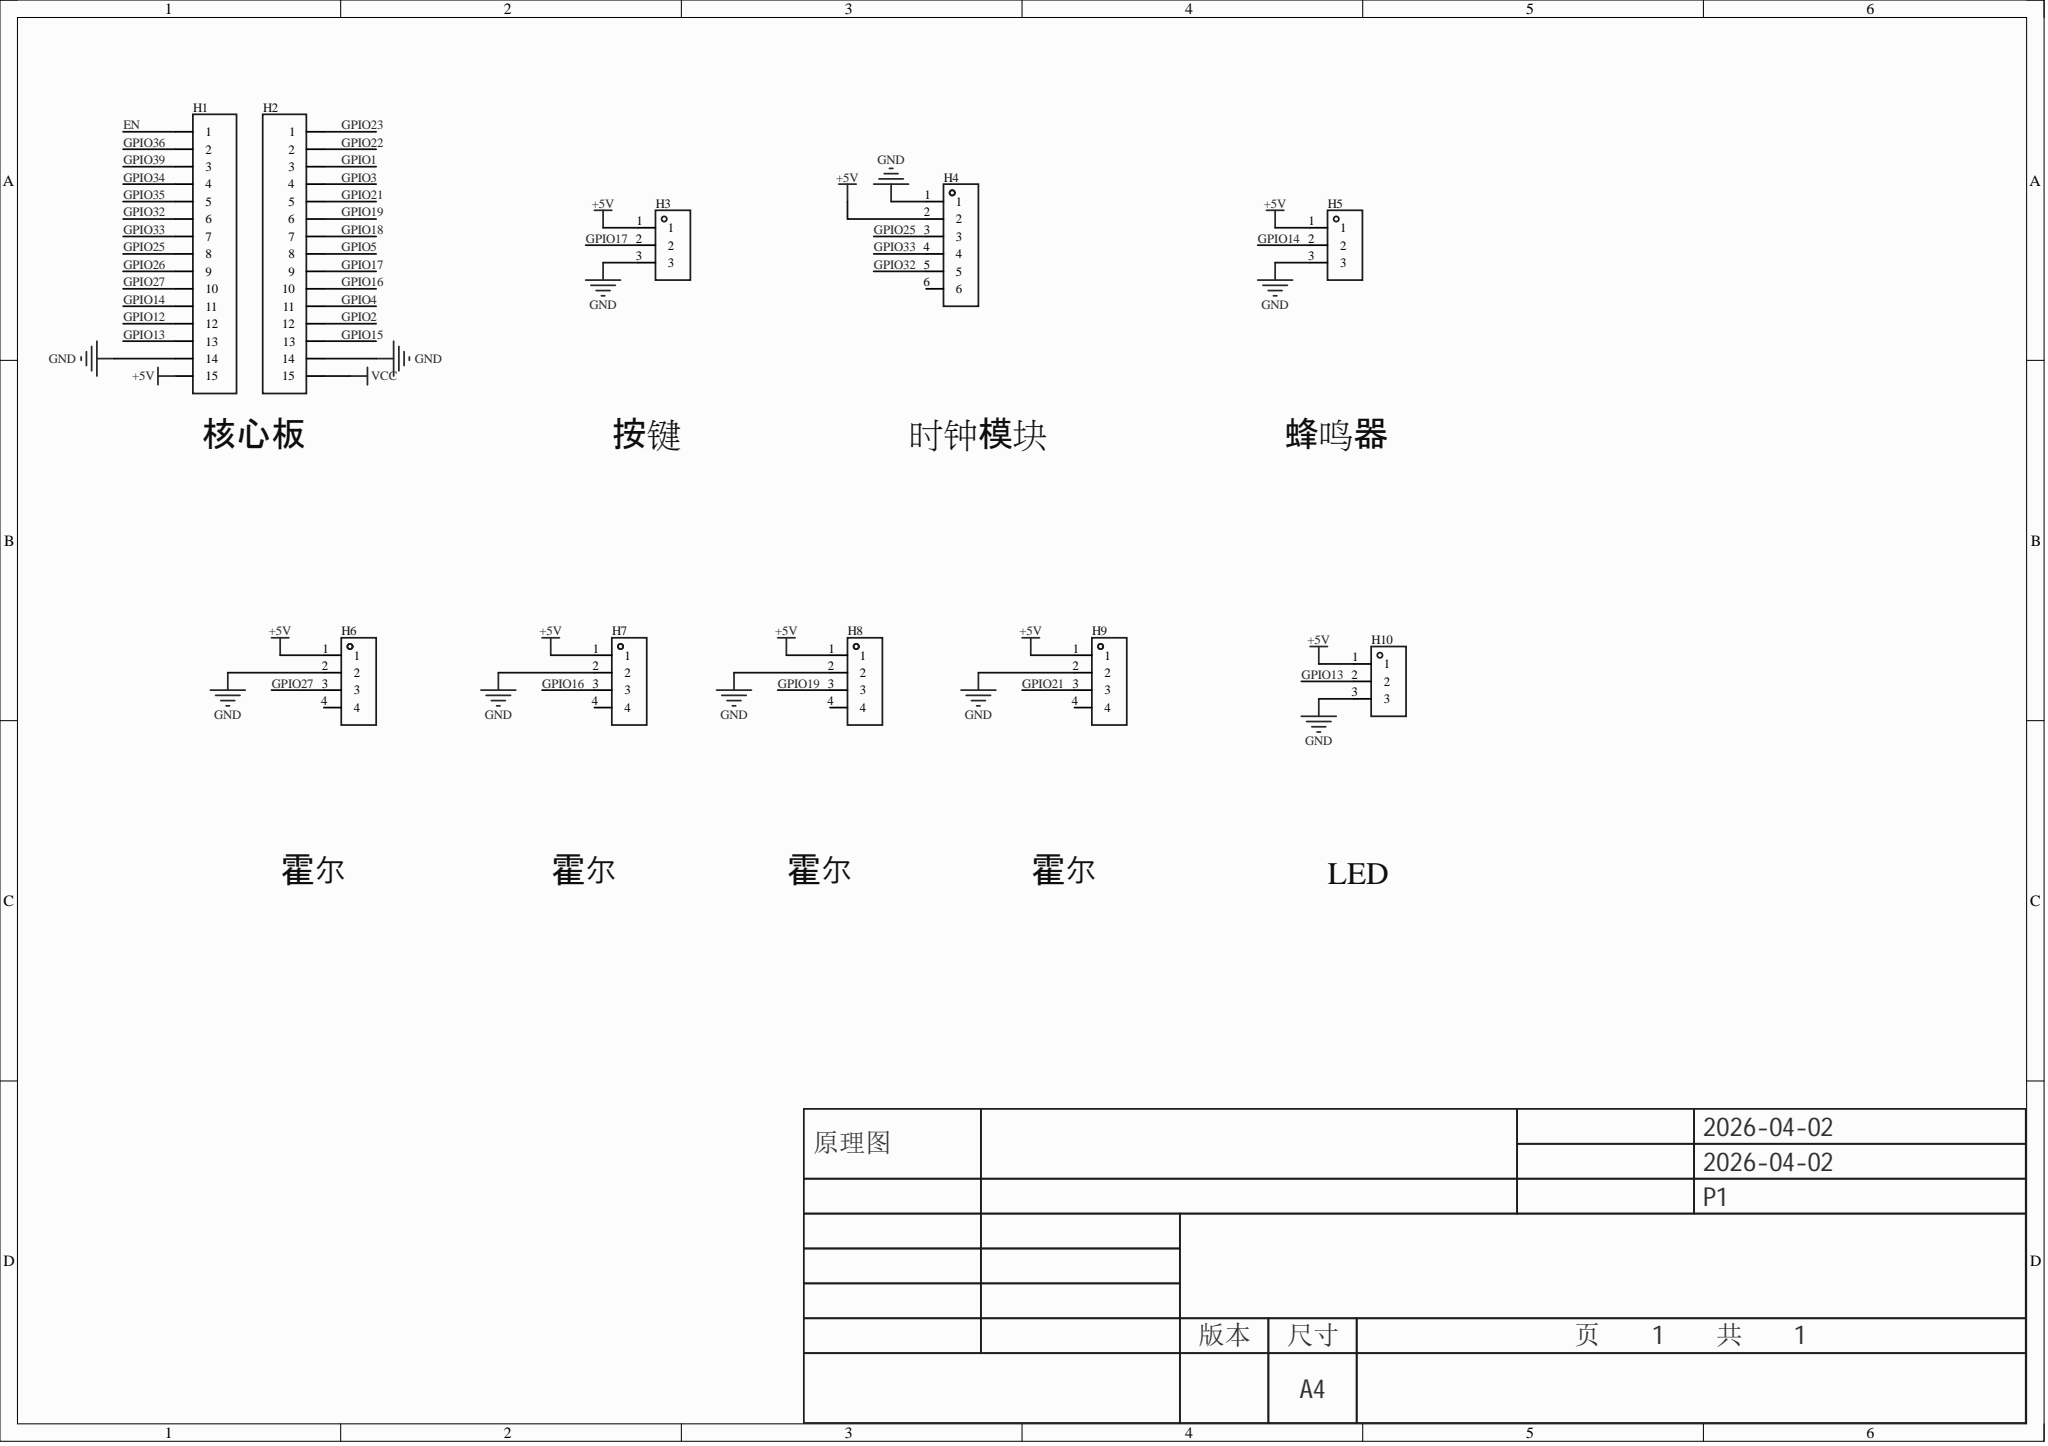Circuit board | Altium Designer | 10 parts | 12 nets
Bill of materials:
Comment,Description,Designator,Footprint,LibRef,Quantity
"","","H1, H2","HDR-TH_15P-P2.54-V-F-1","HDR-F_2.54_1x15P","2"
"","","H3, H5, H10","HDR-TH_3P-P2.54-V-F","HDR-F_2.54_1x3P","3"
"","","H4","HDR-TH_6P-P2.54-V-F","HDR-F_2.54_1x6P","1"
"","","H6, H7, H8, H9","HDR-TH_4P-P2.54-V-F","HDR-F_2.54_1x4P","4"
Netlist (Protel format):
[
H1
HDR-TH_15P-P2.54-V-F-1




]
[
H2
HDR-TH_15P-P2.54-V-F-1




]
[
H3
HDR-TH_3P-P2.54-V-F




]
[
H4
HDR-TH_6P-P2.54-V-F




]
[
H5
HDR-TH_3P-P2.54-V-F




]
[
H6
HDR-TH_4P-P2.54-V-F




]
[
H7
HDR-TH_4P-P2.54-V-F




]
[
H8
HDR-TH_4P-P2.54-V-F




]
[
H9
HDR-TH_4P-P2.54-V-F




]
[
H10
HDR-TH_3P-P2.54-V-F




]
(
GPIO33
H1-7
H4-4
)
(
GPIO32
H1-6
H4-5
)
(
GPIO27
H1-10
H6-3
)
(
GPIO25
H1-8
H4-3
)
(
GPIO21
H2-5
H9-3
)
(
GPIO19
H2-6
H8-3
)
(
GPIO17
H2-9
H3-2
)
(
GPIO16
H2-10
H7-3
)
(
GPIO14
H1-11
H5-2
)
(
GPIO13
H1-13
H10-2
)
(
GND
H1-14
H2-14
H3-3
H4-1
H5-3
H6-2
H7-2
H8-2
H9-2
H10-3
)
(
+5V
H1-15
H3-1
H4-2
H5-1
H6-1
H7-1
H8-1
H9-1
H10-1
)